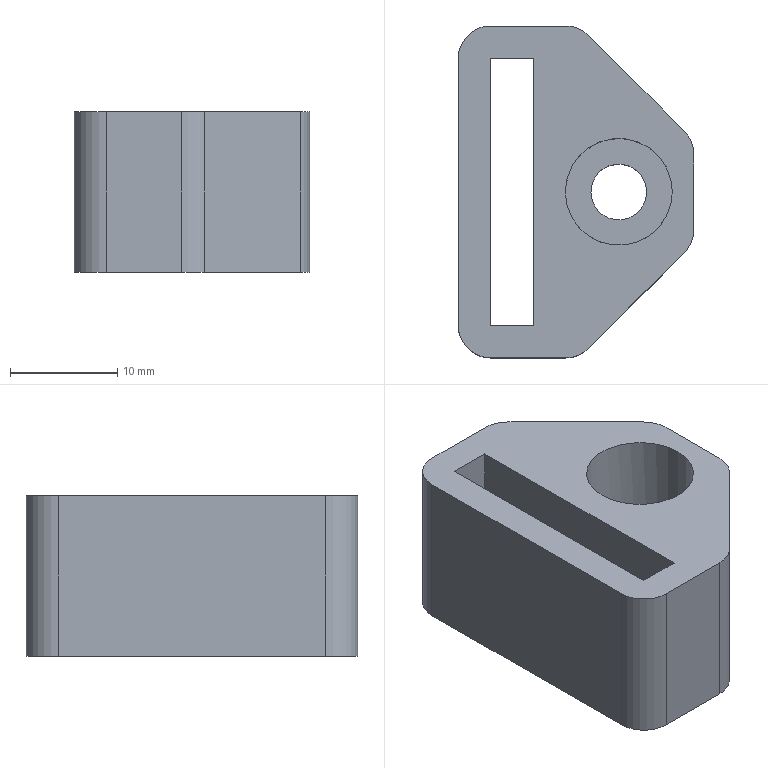Part | NX | features DIE-22 2 | 1 solid | 29 faces | box 22 x 31 x 15 mm | volume 6039 mm3 | plane 17 | cylinder 12 | commonest cylinder face diameters 6 x6 2 x4 5.206 x1 10 x1
STEP:
#1=CARTESIAN_POINT('',(2442.31,-889.273,858.716));
#2=VERTEX_POINT('',#1);
#3=CARTESIAN_POINT('',(2442.31,-864.273,858.716));
#4=VERTEX_POINT('',#3);
#5=CARTESIAN_POINT('',(2442.31,-876.773,858.716));
#6=DIRECTION('',(0.,1.,0.));
#7=VECTOR('',#6,1000.);
#8=LINE('',#5,#7);
#9=EDGE_CURVE('',#2,#4,#8,.T.);
#10=ORIENTED_EDGE('',*,*,#9,.T.);
#11=CARTESIAN_POINT('',(2442.31,-864.273,843.716));
#12=VERTEX_POINT('',#11);
#13=CARTESIAN_POINT('',(2442.31,-864.273,840.716));
#14=DIRECTION('',(0.,0.,1.));
#15=VECTOR('',#14,1000.);
#16=LINE('',#13,#15);
#17=EDGE_CURVE('',#4,#12,#16,.F.);
#18=ORIENTED_EDGE('',*,*,#17,.T.);
#19=CARTESIAN_POINT('',(2442.31,-889.273,843.716));
#20=VERTEX_POINT('',#19);
#21=CARTESIAN_POINT('',(2442.31,-876.773,843.716));
#22=DIRECTION('',(0.,-1.,0.));
#23=VECTOR('',#22,1000.);
#24=LINE('',#21,#23);
#25=EDGE_CURVE('',#12,#20,#24,.T.);
#26=ORIENTED_EDGE('',*,*,#25,.T.);
#27=CARTESIAN_POINT('',(2442.31,-889.273,840.716));
#28=DIRECTION('',(0.,0.,1.));
#29=VECTOR('',#28,1000.);
#30=LINE('',#27,#29);
#31=EDGE_CURVE('',#20,#2,#30,.T.);
#32=ORIENTED_EDGE('',*,*,#31,.T.);
#33=EDGE_LOOP('',(#10,#18,#26,#32));
#34=FACE_BOUND('',#33,.T.);
#35=CARTESIAN_POINT('',(2442.31,-876.773,840.716));
#36=DIRECTION('',(-1.,0.,0.));
#37=DIRECTION('',(0.,0.,1.));
#38=AXIS2_PLACEMENT_3D('',#35,#36,#37);
#39=PLANE('',#38);
#40=ADVANCED_FACE('',(#34),#39,.T.);
#41=CARTESIAN_POINT('',(2445.31,-892.273,843.716));
#42=VERTEX_POINT('',#41);
#43=CARTESIAN_POINT('',(2445.31,-889.273,843.716));
#44=DIRECTION('',(0.,0.,-1.));
#45=DIRECTION('',(-1.,0.,0.));
#46=AXIS2_PLACEMENT_3D('',#43,#44,#45);
#47=CIRCLE('',#46,3.);
#48=EDGE_CURVE('',#42,#20,#47,.T.);
#49=ORIENTED_EDGE('',*,*,#48,.F.);
#50=CARTESIAN_POINT('',(2445.31,-892.273,858.716));
#51=VERTEX_POINT('',#50);
#52=CARTESIAN_POINT('',(2445.31,-892.273,840.716));
#53=DIRECTION('',(0.,0.,1.));
#54=VECTOR('',#53,1000.);
#55=LINE('',#52,#54);
#56=EDGE_CURVE('',#51,#42,#55,.F.);
#57=ORIENTED_EDGE('',*,*,#56,.F.);
#58=CARTESIAN_POINT('',(2445.31,-889.273,858.716));
#59=DIRECTION('',(0.,0.,1.));
#60=DIRECTION('',(1.,0.,0.));
#61=AXIS2_PLACEMENT_3D('',#58,#59,#60);
#62=CIRCLE('',#61,3.);
#63=EDGE_CURVE('',#2,#51,#62,.T.);
#64=ORIENTED_EDGE('',*,*,#63,.F.);
#65=ORIENTED_EDGE('',*,*,#31,.F.);
#66=EDGE_LOOP('',(#49,#57,#64,#65));
#67=FACE_BOUND('',#66,.T.);
#68=CARTESIAN_POINT('',(2445.31,-889.273,840.716));
#69=DIRECTION('',(0.,0.,1.));
#70=DIRECTION('',(1.,0.,0.));
#71=AXIS2_PLACEMENT_3D('',#68,#69,#70);
#72=CYLINDRICAL_SURFACE('',#71,3.);
#73=ADVANCED_FACE('',(#67),#72,.T.);
#74=CARTESIAN_POINT('',(2445.31,-861.273,843.716));
#75=VERTEX_POINT('',#74);
#76=CARTESIAN_POINT('',(2445.31,-864.273,843.716));
#77=DIRECTION('',(0.,0.,-1.));
#78=DIRECTION('',(-1.,0.,0.));
#79=AXIS2_PLACEMENT_3D('',#76,#77,#78);
#80=CIRCLE('',#79,3.);
#81=EDGE_CURVE('',#12,#75,#80,.T.);
#82=ORIENTED_EDGE('',*,*,#81,.F.);
#83=ORIENTED_EDGE('',*,*,#17,.F.);
#84=CARTESIAN_POINT('',(2445.31,-861.273,858.716));
#85=VERTEX_POINT('',#84);
#86=CARTESIAN_POINT('',(2445.31,-864.273,858.716));
#87=DIRECTION('',(0.,0.,1.));
#88=DIRECTION('',(1.,0.,0.));
#89=AXIS2_PLACEMENT_3D('',#86,#87,#88);
#90=CIRCLE('',#89,3.);
#91=EDGE_CURVE('',#85,#4,#90,.T.);
#92=ORIENTED_EDGE('',*,*,#91,.F.);
#93=CARTESIAN_POINT('',(2445.31,-861.273,840.716));
#94=DIRECTION('',(0.,0.,1.));
#95=VECTOR('',#94,1000.);
#96=LINE('',#93,#95);
#97=EDGE_CURVE('',#75,#85,#96,.T.);
#98=ORIENTED_EDGE('',*,*,#97,.F.);
#99=EDGE_LOOP('',(#82,#83,#92,#98));
#100=FACE_BOUND('',#99,.T.);
#101=CARTESIAN_POINT('',(2445.31,-864.273,840.716));
#102=DIRECTION('',(0.,0.,1.));
#103=DIRECTION('',(1.,0.,0.));
#104=AXIS2_PLACEMENT_3D('',#101,#102,#103);
#105=CYLINDRICAL_SURFACE('',#104,3.);
#106=ADVANCED_FACE('',(#100),#105,.T.);
#107=CARTESIAN_POINT('',(2445.31,-864.273,858.716));
#108=VERTEX_POINT('',#107);
#109=CARTESIAN_POINT('',(2445.31,-889.273,858.716));
#110=VERTEX_POINT('',#109);
#111=CARTESIAN_POINT('',(2445.31,-885.523,858.716));
#112=DIRECTION('',(0.,-1.,0.));
#113=VECTOR('',#112,1000.);
#114=LINE('',#111,#113);
#115=EDGE_CURVE('',#108,#110,#114,.T.);
#116=ORIENTED_EDGE('',*,*,#115,.T.);
#117=CARTESIAN_POINT('',(2445.31,-889.273,843.716));
#118=VERTEX_POINT('',#117);
#119=CARTESIAN_POINT('',(2445.31,-889.273,858.516));
#120=DIRECTION('',(0.,0.,-1.));
#121=VECTOR('',#120,1000.);
#122=LINE('',#119,#121);
#123=EDGE_CURVE('',#118,#110,#122,.F.);
#124=ORIENTED_EDGE('',*,*,#123,.F.);
#125=CARTESIAN_POINT('',(2445.31,-864.273,843.716));
#126=VERTEX_POINT('',#125);
#127=CARTESIAN_POINT('',(2445.31,-884.898,843.716));
#128=DIRECTION('',(0.,-1.,0.));
#129=VECTOR('',#128,1000.);
#130=LINE('',#127,#129);
#131=EDGE_CURVE('',#126,#118,#130,.T.);
#132=ORIENTED_EDGE('',*,*,#131,.F.);
#133=CARTESIAN_POINT('',(2445.31,-864.273,858.516));
#134=DIRECTION('',(0.,0.,-1.));
#135=VECTOR('',#134,1000.);
#136=LINE('',#133,#135);
#137=EDGE_CURVE('',#108,#126,#136,.T.);
#138=ORIENTED_EDGE('',*,*,#137,.F.);
#139=EDGE_LOOP('',(#116,#124,#132,#138));
#140=FACE_BOUND('',#139,.T.);
#141=CARTESIAN_POINT('',(2445.31,-884.898,858.516));
#142=DIRECTION('',(1.,0.,0.));
#143=DIRECTION('',(0.,0.,1.));
#144=AXIS2_PLACEMENT_3D('',#141,#142,#143);
#145=PLANE('',#144);
#146=ADVANCED_FACE('',(#140),#145,.T.);
#147=CARTESIAN_POINT('',(2448.31,-889.273,843.716));
#148=VERTEX_POINT('',#147);
#149=CARTESIAN_POINT('',(2448.31,-889.273,846.716));
#150=VERTEX_POINT('',#149);
#151=CARTESIAN_POINT('',(2448.31,-889.273,858.516));
#152=DIRECTION('',(0.,0.,1.));
#153=VECTOR('',#152,1000.);
#154=LINE('',#151,#153);
#155=EDGE_CURVE('',#148,#150,#154,.T.);
#156=ORIENTED_EDGE('',*,*,#155,.F.);
#157=CARTESIAN_POINT('',(2448.697,-889.273,843.716));
#158=DIRECTION('',(1.,0.,0.));
#159=VECTOR('',#158,1000.);
#160=LINE('',#157,#159);
#161=EDGE_CURVE('',#118,#148,#160,.T.);
#162=ORIENTED_EDGE('',*,*,#161,.F.);
#163=ORIENTED_EDGE('',*,*,#123,.T.);
#164=CARTESIAN_POINT('',(2449.31,-889.273,858.716));
#165=VERTEX_POINT('',#164);
#166=CARTESIAN_POINT('',(2447.31,-889.273,858.716));
#167=DIRECTION('',(1.,0.,0.));
#168=VECTOR('',#167,1000.);
#169=LINE('',#166,#168);
#170=EDGE_CURVE('',#165,#110,#169,.F.);
#171=ORIENTED_EDGE('',*,*,#170,.F.);
#172=CARTESIAN_POINT('',(2449.31,-889.273,846.716));
#173=VERTEX_POINT('',#172);
#174=CARTESIAN_POINT('',(2449.31,-889.273,858.516));
#175=DIRECTION('',(0.,0.,1.));
#176=VECTOR('',#175,1000.);
#177=LINE('',#174,#176);
#178=EDGE_CURVE('',#173,#165,#177,.T.);
#179=ORIENTED_EDGE('',*,*,#178,.F.);
#180=CARTESIAN_POINT('',(2449.81,-889.273,846.716));
#181=DIRECTION('',(-1.,0.,0.));
#182=VECTOR('',#181,1000.);
#183=LINE('',#180,#182);
#184=EDGE_CURVE('',#173,#150,#183,.T.);
#185=ORIENTED_EDGE('',*,*,#184,.T.);
#186=EDGE_LOOP('',(#156,#162,#163,#171,#179,#185));
#187=FACE_BOUND('',#186,.T.);
#188=CARTESIAN_POINT('',(2448.697,-889.273,858.516));
#189=DIRECTION('',(0.,1.,0.));
#190=DIRECTION('',(0.,0.,-1.));
#191=AXIS2_PLACEMENT_3D('',#188,#189,#190);
#192=PLANE('',#191);
#193=ADVANCED_FACE('',(#187),#192,.T.);
#194=CARTESIAN_POINT('',(2448.31,-864.273,843.716));
#195=VERTEX_POINT('',#194);
#196=CARTESIAN_POINT('',(2448.697,-864.273,843.716));
#197=DIRECTION('',(-1.,0.,0.));
#198=VECTOR('',#197,1000.);
#199=LINE('',#196,#198);
#200=EDGE_CURVE('',#195,#126,#199,.T.);
#201=ORIENTED_EDGE('',*,*,#200,.F.);
#202=CARTESIAN_POINT('',(2448.31,-864.273,846.716));
#203=VERTEX_POINT('',#202);
#204=CARTESIAN_POINT('',(2448.31,-864.273,858.516));
#205=DIRECTION('',(0.,0.,-1.));
#206=VECTOR('',#205,1000.);
#207=LINE('',#204,#206);
#208=EDGE_CURVE('',#203,#195,#207,.T.);
#209=ORIENTED_EDGE('',*,*,#208,.F.);
#210=CARTESIAN_POINT('',(2449.31,-864.273,846.716));
#211=VERTEX_POINT('',#210);
#212=CARTESIAN_POINT('',(2448.697,-864.273,846.716));
#213=DIRECTION('',(-1.,0.,0.));
#214=VECTOR('',#213,1000.);
#215=LINE('',#212,#214);
#216=EDGE_CURVE('',#211,#203,#215,.T.);
#217=ORIENTED_EDGE('',*,*,#216,.F.);
#218=CARTESIAN_POINT('',(2449.31,-864.273,858.716));
#219=VERTEX_POINT('',#218);
#220=CARTESIAN_POINT('',(2449.31,-864.273,858.516));
#221=DIRECTION('',(0.,0.,-1.));
#222=VECTOR('',#221,1000.);
#223=LINE('',#220,#222);
#224=EDGE_CURVE('',#219,#211,#223,.T.);
#225=ORIENTED_EDGE('',*,*,#224,.F.);
#226=CARTESIAN_POINT('',(2447.31,-864.273,858.716));
#227=DIRECTION('',(1.,0.,0.));
#228=VECTOR('',#227,1000.);
#229=LINE('',#226,#228);
#230=EDGE_CURVE('',#219,#108,#229,.F.);
#231=ORIENTED_EDGE('',*,*,#230,.T.);
#232=ORIENTED_EDGE('',*,*,#137,.T.);
#233=EDGE_LOOP('',(#201,#209,#217,#225,#231,#232));
#234=FACE_BOUND('',#233,.T.);
#235=CARTESIAN_POINT('',(2448.697,-864.273,858.516));
#236=DIRECTION('',(0.,-1.,0.));
#237=DIRECTION('',(0.,0.,-1.));
#238=AXIS2_PLACEMENT_3D('',#235,#236,#237);
#239=PLANE('',#238);
#240=ADVANCED_FACE('',(#234),#239,.T.);
#241=CARTESIAN_POINT('',(2452.36,-861.273,858.716));
#242=VERTEX_POINT('',#241);
#243=CARTESIAN_POINT('',(2447.81,-861.273,858.716));
#244=DIRECTION('',(1.,0.,0.));
#245=VECTOR('',#244,1000.);
#246=LINE('',#243,#245);
#247=EDGE_CURVE('',#85,#242,#246,.T.);
#248=ORIENTED_EDGE('',*,*,#247,.T.);
#249=CARTESIAN_POINT('',(2452.36,-861.273,843.716));
#250=VERTEX_POINT('',#249);
#251=CARTESIAN_POINT('',(2452.36,-861.273,840.716));
#252=DIRECTION('',(0.,0.,1.));
#253=VECTOR('',#252,1000.);
#254=LINE('',#251,#253);
#255=EDGE_CURVE('',#242,#250,#254,.F.);
#256=ORIENTED_EDGE('',*,*,#255,.T.);
#257=CARTESIAN_POINT('',(2447.81,-861.273,843.716));
#258=DIRECTION('',(-1.,0.,0.));
#259=VECTOR('',#258,1000.);
#260=LINE('',#257,#259);
#261=EDGE_CURVE('',#250,#75,#260,.T.);
#262=ORIENTED_EDGE('',*,*,#261,.T.);
#263=ORIENTED_EDGE('',*,*,#97,.T.);
#264=EDGE_LOOP('',(#248,#256,#262,#263));
#265=FACE_BOUND('',#264,.T.);
#266=CARTESIAN_POINT('',(2447.81,-861.273,840.716));
#267=DIRECTION('',(0.,1.,0.));
#268=DIRECTION('',(0.,0.,1.));
#269=AXIS2_PLACEMENT_3D('',#266,#267,#268);
#270=PLANE('',#269);
#271=ADVANCED_FACE('',(#265),#270,.T.);
#272=CARTESIAN_POINT('',(2452.36,-892.273,843.716));
#273=VERTEX_POINT('',#272);
#274=CARTESIAN_POINT('',(2447.81,-892.273,843.716));
#275=DIRECTION('',(1.,0.,0.));
#276=VECTOR('',#275,1000.);
#277=LINE('',#274,#276);
#278=EDGE_CURVE('',#42,#273,#277,.T.);
#279=ORIENTED_EDGE('',*,*,#278,.T.);
#280=CARTESIAN_POINT('',(2452.36,-892.273,858.716));
#281=VERTEX_POINT('',#280);
#282=CARTESIAN_POINT('',(2452.36,-892.273,840.716));
#283=DIRECTION('',(0.,0.,-1.));
#284=VECTOR('',#283,1000.);
#285=LINE('',#282,#284);
#286=EDGE_CURVE('',#273,#281,#285,.F.);
#287=ORIENTED_EDGE('',*,*,#286,.T.);
#288=CARTESIAN_POINT('',(2447.81,-892.273,858.716));
#289=DIRECTION('',(-1.,0.,0.));
#290=VECTOR('',#289,1000.);
#291=LINE('',#288,#290);
#292=EDGE_CURVE('',#281,#51,#291,.T.);
#293=ORIENTED_EDGE('',*,*,#292,.T.);
#294=ORIENTED_EDGE('',*,*,#56,.T.);
#295=EDGE_LOOP('',(#279,#287,#293,#294));
#296=FACE_BOUND('',#295,.T.);
#297=CARTESIAN_POINT('',(2447.81,-892.273,840.716));
#298=DIRECTION('',(0.,-1.,0.));
#299=DIRECTION('',(0.,0.,-1.));
#300=AXIS2_PLACEMENT_3D('',#297,#298,#299);
#301=PLANE('',#300);
#302=ADVANCED_FACE('',(#296),#301,.T.);
#303=ORIENTED_EDGE('',*,*,#161,.T.);
#304=CARTESIAN_POINT('',(2449.31,-890.273,843.716));
#305=VERTEX_POINT('',#304);
#306=CARTESIAN_POINT('',(2449.31,-889.273,843.716));
#307=DIRECTION('',(0.,0.,-1.));
#308=DIRECTION('',(-1.,0.,0.));
#309=AXIS2_PLACEMENT_3D('',#306,#307,#308);
#310=CIRCLE('',#309,1.);
#311=EDGE_CURVE('',#148,#305,#310,.F.);
#312=ORIENTED_EDGE('',*,*,#311,.T.);
#313=CARTESIAN_POINT('',(2449.81,-890.273,843.716));
#314=VERTEX_POINT('',#313);
#315=CARTESIAN_POINT('',(2447.81,-890.273,843.716));
#316=DIRECTION('',(1.,0.,0.));
#317=VECTOR('',#316,1000.);
#318=LINE('',#315,#317);
#319=EDGE_CURVE('',#305,#314,#318,.T.);
#320=ORIENTED_EDGE('',*,*,#319,.T.);
#321=CARTESIAN_POINT('',(2450.81,-889.273,843.716));
#322=VERTEX_POINT('',#321);
#323=CARTESIAN_POINT('',(2449.81,-889.273,843.716));
#324=DIRECTION('',(0.,0.,-1.));
#325=DIRECTION('',(-1.,0.,0.));
#326=AXIS2_PLACEMENT_3D('',#323,#324,#325);
#327=CIRCLE('',#326,1.);
#328=EDGE_CURVE('',#314,#322,#327,.F.);
#329=ORIENTED_EDGE('',*,*,#328,.T.);
#330=CARTESIAN_POINT('',(2450.81,-864.273,843.716));
#331=VERTEX_POINT('',#330);
#332=CARTESIAN_POINT('',(2450.81,-884.898,843.716));
#333=DIRECTION('',(0.,-1.,0.));
#334=VECTOR('',#333,1000.);
#335=LINE('',#332,#334);
#336=EDGE_CURVE('',#331,#322,#335,.T.);
#337=ORIENTED_EDGE('',*,*,#336,.F.);
#338=CARTESIAN_POINT('',(2449.81,-863.273,843.716));
#339=VERTEX_POINT('',#338);
#340=CARTESIAN_POINT('',(2449.81,-864.273,843.716));
#341=DIRECTION('',(0.,0.,-1.));
#342=DIRECTION('',(-1.,0.,0.));
#343=AXIS2_PLACEMENT_3D('',#340,#341,#342);
#344=CIRCLE('',#343,1.);
#345=EDGE_CURVE('',#331,#339,#344,.F.);
#346=ORIENTED_EDGE('',*,*,#345,.T.);
#347=CARTESIAN_POINT('',(2449.31,-863.273,843.716));
#348=VERTEX_POINT('',#347);
#349=CARTESIAN_POINT('',(2447.81,-863.273,843.716));
#350=DIRECTION('',(-1.,0.,0.));
#351=VECTOR('',#350,1000.);
#352=LINE('',#349,#351);
#353=EDGE_CURVE('',#339,#348,#352,.T.);
#354=ORIENTED_EDGE('',*,*,#353,.T.);
#355=CARTESIAN_POINT('',(2449.31,-864.273,843.716));
#356=DIRECTION('',(0.,0.,-1.));
#357=DIRECTION('',(-1.,0.,0.));
#358=AXIS2_PLACEMENT_3D('',#355,#356,#357);
#359=CIRCLE('',#358,1.);
#360=EDGE_CURVE('',#348,#195,#359,.F.);
#361=ORIENTED_EDGE('',*,*,#360,.T.);
#362=ORIENTED_EDGE('',*,*,#200,.T.);
#363=ORIENTED_EDGE('',*,*,#131,.T.);
#364=EDGE_LOOP('',(#303,#312,#320,#329,#337,#346,#354,#361,#362,#363));
#365=FACE_BOUND('',#364,.T.);
#366=CARTESIAN_POINT('',(2454.481,-891.395,843.716));
#367=VERTEX_POINT('',#366);
#368=CARTESIAN_POINT('',(2452.36,-889.273,843.716));
#369=DIRECTION('',(0.,0.,-1.));
#370=DIRECTION('',(-1.,0.,0.));
#371=AXIS2_PLACEMENT_3D('',#368,#369,#370);
#372=CIRCLE('',#371,3.);
#373=EDGE_CURVE('',#367,#273,#372,.T.);
#374=ORIENTED_EDGE('',*,*,#373,.T.);
#375=ORIENTED_EDGE('',*,*,#278,.F.);
#376=ORIENTED_EDGE('',*,*,#48,.T.);
#377=ORIENTED_EDGE('',*,*,#25,.F.);
#378=ORIENTED_EDGE('',*,*,#81,.T.);
#379=ORIENTED_EDGE('',*,*,#261,.F.);
#380=CARTESIAN_POINT('',(2454.481,-862.152,843.716));
#381=VERTEX_POINT('',#380);
#382=CARTESIAN_POINT('',(2452.36,-864.273,843.716));
#383=DIRECTION('',(0.,0.,-1.));
#384=DIRECTION('',(-1.,0.,0.));
#385=AXIS2_PLACEMENT_3D('',#382,#383,#384);
#386=CIRCLE('',#385,3.);
#387=EDGE_CURVE('',#250,#381,#386,.T.);
#388=ORIENTED_EDGE('',*,*,#387,.T.);
#389=CARTESIAN_POINT('',(2463.431,-871.102,843.716));
#390=VERTEX_POINT('',#389);
#391=CARTESIAN_POINT('',(2458.456,-866.127,843.716));
#392=DIRECTION('',(-0.7071,0.7071,0.));
#393=VECTOR('',#392,1000.);
#394=LINE('',#391,#393);
#395=EDGE_CURVE('',#381,#390,#394,.F.);
#396=ORIENTED_EDGE('',*,*,#395,.T.);
#397=CARTESIAN_POINT('',(2464.31,-873.223,843.716));
#398=VERTEX_POINT('',#397);
#399=CARTESIAN_POINT('',(2461.31,-873.223,843.716));
#400=DIRECTION('',(0.,0.,-1.));
#401=DIRECTION('',(-1.,0.,0.));
#402=AXIS2_PLACEMENT_3D('',#399,#400,#401);
#403=CIRCLE('',#402,3.);
#404=EDGE_CURVE('',#390,#398,#403,.T.);
#405=ORIENTED_EDGE('',*,*,#404,.T.);
#406=CARTESIAN_POINT('',(2464.31,-880.324,843.716));
#407=VERTEX_POINT('',#406);
#408=CARTESIAN_POINT('',(2464.31,-876.773,843.716));
#409=DIRECTION('',(0.,1.,0.));
#410=VECTOR('',#409,1000.);
#411=LINE('',#408,#410);
#412=EDGE_CURVE('',#407,#398,#411,.T.);
#413=ORIENTED_EDGE('',*,*,#412,.F.);
#414=CARTESIAN_POINT('',(2463.431,-882.445,843.716));
#415=VERTEX_POINT('',#414);
#416=CARTESIAN_POINT('',(2461.31,-880.324,843.716));
#417=DIRECTION('',(0.,0.,-1.));
#418=DIRECTION('',(-1.,0.,0.));
#419=AXIS2_PLACEMENT_3D('',#416,#417,#418);
#420=CIRCLE('',#419,3.);
#421=EDGE_CURVE('',#407,#415,#420,.T.);
#422=ORIENTED_EDGE('',*,*,#421,.T.);
#423=CARTESIAN_POINT('',(2458.456,-887.42,843.716));
#424=DIRECTION('',(0.7071,0.7071,0.));
#425=VECTOR('',#424,1000.);
#426=LINE('',#423,#425);
#427=EDGE_CURVE('',#415,#367,#426,.F.);
#428=ORIENTED_EDGE('',*,*,#427,.T.);
#429=EDGE_LOOP('',(#374,#375,#376,#377,#378,#379,#388,#396,#405,#413,#422,#428));
#430=FACE_BOUND('',#429,.T.);
#431=CARTESIAN_POINT('',(2454.707,-876.773,843.716));
#432=VERTEX_POINT('',#431);
#433=CARTESIAN_POINT('',(2457.31,-876.773,843.716));
#434=DIRECTION('',(0.,0.,-1.));
#435=DIRECTION('',(-1.,0.,0.));
#436=AXIS2_PLACEMENT_3D('',#433,#434,#435);
#437=CIRCLE('',#436,2.603);
#438=EDGE_CURVE('',#432,#432,#437,.T.);
#439=ORIENTED_EDGE('',*,*,#438,.F.);
#440=EDGE_LOOP('',(#439));
#441=FACE_BOUND('',#440,.T.);
#442=CARTESIAN_POINT('',(2447.81,-876.773,843.716));
#443=DIRECTION('',(0.,0.,-1.));
#444=DIRECTION('',(-1.,0.,0.));
#445=AXIS2_PLACEMENT_3D('',#442,#443,#444);
#446=PLANE('',#445);
#447=ADVANCED_FACE('',(#365,#430,#441),#446,.T.);
#448=ORIENTED_EDGE('',*,*,#230,.F.);
#449=CARTESIAN_POINT('',(2449.31,-876.773,858.716));
#450=DIRECTION('',(0.,-1.,0.));
#451=VECTOR('',#450,1000.);
#452=LINE('',#449,#451);
#453=EDGE_CURVE('',#165,#219,#452,.F.);
#454=ORIENTED_EDGE('',*,*,#453,.F.);
#455=ORIENTED_EDGE('',*,*,#170,.T.);
#456=ORIENTED_EDGE('',*,*,#115,.F.);
#457=EDGE_LOOP('',(#448,#454,#455,#456));
#458=FACE_BOUND('',#457,.T.);
#459=CARTESIAN_POINT('',(2454.481,-862.152,858.716));
#460=VERTEX_POINT('',#459);
#461=CARTESIAN_POINT('',(2452.36,-864.273,858.716));
#462=DIRECTION('',(0.,0.,1.));
#463=DIRECTION('',(1.,0.,0.));
#464=AXIS2_PLACEMENT_3D('',#461,#462,#463);
#465=CIRCLE('',#464,3.);
#466=EDGE_CURVE('',#460,#242,#465,.T.);
#467=ORIENTED_EDGE('',*,*,#466,.T.);
#468=ORIENTED_EDGE('',*,*,#247,.F.);
#469=ORIENTED_EDGE('',*,*,#91,.T.);
#470=ORIENTED_EDGE('',*,*,#9,.F.);
#471=ORIENTED_EDGE('',*,*,#63,.T.);
#472=ORIENTED_EDGE('',*,*,#292,.F.);
#473=CARTESIAN_POINT('',(2454.481,-891.395,858.716));
#474=VERTEX_POINT('',#473);
#475=CARTESIAN_POINT('',(2452.36,-889.273,858.716));
#476=DIRECTION('',(0.,0.,1.));
#477=DIRECTION('',(1.,0.,0.));
#478=AXIS2_PLACEMENT_3D('',#475,#476,#477);
#479=CIRCLE('',#478,3.);
#480=EDGE_CURVE('',#281,#474,#479,.T.);
#481=ORIENTED_EDGE('',*,*,#480,.T.);
#482=CARTESIAN_POINT('',(2463.431,-882.445,858.716));
#483=VERTEX_POINT('',#482);
#484=CARTESIAN_POINT('',(2458.456,-887.42,858.716));
#485=DIRECTION('',(-0.7071,-0.7071,0.));
#486=VECTOR('',#485,1000.);
#487=LINE('',#484,#486);
#488=EDGE_CURVE('',#474,#483,#487,.F.);
#489=ORIENTED_EDGE('',*,*,#488,.T.);
#490=CARTESIAN_POINT('',(2464.31,-880.324,858.716));
#491=VERTEX_POINT('',#490);
#492=CARTESIAN_POINT('',(2461.31,-880.324,858.716));
#493=DIRECTION('',(0.,0.,1.));
#494=DIRECTION('',(1.,0.,0.));
#495=AXIS2_PLACEMENT_3D('',#492,#493,#494);
#496=CIRCLE('',#495,3.);
#497=EDGE_CURVE('',#483,#491,#496,.T.);
#498=ORIENTED_EDGE('',*,*,#497,.T.);
#499=CARTESIAN_POINT('',(2464.31,-873.223,858.716));
#500=VERTEX_POINT('',#499);
#501=CARTESIAN_POINT('',(2464.31,-876.773,858.716));
#502=DIRECTION('',(0.,-1.,0.));
#503=VECTOR('',#502,1000.);
#504=LINE('',#501,#503);
#505=EDGE_CURVE('',#500,#491,#504,.T.);
#506=ORIENTED_EDGE('',*,*,#505,.F.);
#507=CARTESIAN_POINT('',(2463.431,-871.102,858.716));
#508=VERTEX_POINT('',#507);
#509=CARTESIAN_POINT('',(2461.31,-873.223,858.716));
#510=DIRECTION('',(0.,0.,1.));
#511=DIRECTION('',(1.,0.,0.));
#512=AXIS2_PLACEMENT_3D('',#509,#510,#511);
#513=CIRCLE('',#512,3.);
#514=EDGE_CURVE('',#500,#508,#513,.T.);
#515=ORIENTED_EDGE('',*,*,#514,.T.);
#516=CARTESIAN_POINT('',(2458.456,-866.127,858.716));
#517=DIRECTION('',(0.7071,-0.7071,0.));
#518=VECTOR('',#517,1000.);
#519=LINE('',#516,#518);
#520=EDGE_CURVE('',#508,#460,#519,.F.);
#521=ORIENTED_EDGE('',*,*,#520,.T.);
#522=EDGE_LOOP('',(#467,#468,#469,#470,#471,#472,#481,#489,#498,#506,#515,#521));
#523=FACE_BOUND('',#522,.T.);
#524=CARTESIAN_POINT('',(2462.31,-876.773,858.716));
#525=VERTEX_POINT('',#524);
#526=CARTESIAN_POINT('',(2457.31,-876.773,858.716));
#527=DIRECTION('',(0.,0.,1.));
#528=DIRECTION('',(1.,0.,0.));
#529=AXIS2_PLACEMENT_3D('',#526,#527,#528);
#530=CIRCLE('',#529,5.);
#531=EDGE_CURVE('',#525,#525,#530,.T.);
#532=ORIENTED_EDGE('',*,*,#531,.F.);
#533=EDGE_LOOP('',(#532));
#534=FACE_BOUND('',#533,.T.);
#535=CARTESIAN_POINT('',(2447.81,-876.773,858.716));
#536=DIRECTION('',(0.,0.,1.));
#537=DIRECTION('',(1.,0.,0.));
#538=AXIS2_PLACEMENT_3D('',#535,#536,#537);
#539=PLANE('',#538);
#540=ADVANCED_FACE('',(#458,#523,#534),#539,.T.);
#541=ORIENTED_EDGE('',*,*,#319,.F.);
#542=CARTESIAN_POINT('',(2449.31,-890.273,846.716));
#543=VERTEX_POINT('',#542);
#544=CARTESIAN_POINT('',(2449.31,-890.273,858.516));
#545=DIRECTION('',(0.,0.,-1.));
#546=VECTOR('',#545,1000.);
#547=LINE('',#544,#546);
#548=EDGE_CURVE('',#305,#543,#547,.F.);
#549=ORIENTED_EDGE('',*,*,#548,.T.);
#550=CARTESIAN_POINT('',(2449.81,-890.273,846.716));
#551=VERTEX_POINT('',#550);
#552=CARTESIAN_POINT('',(2449.81,-890.273,846.716));
#553=DIRECTION('',(-1.,0.,0.));
#554=VECTOR('',#553,1000.);
#555=LINE('',#552,#554);
#556=EDGE_CURVE('',#551,#543,#555,.T.);
#557=ORIENTED_EDGE('',*,*,#556,.F.);
#558=CARTESIAN_POINT('',(2449.81,-890.273,843.716));
#559=DIRECTION('',(0.,0.,1.));
#560=VECTOR('',#559,1000.);
#561=LINE('',#558,#560);
#562=EDGE_CURVE('',#551,#314,#561,.F.);
#563=ORIENTED_EDGE('',*,*,#562,.T.);
#564=EDGE_LOOP('',(#541,#549,#557,#563));
#565=FACE_BOUND('',#564,.T.);
#566=CARTESIAN_POINT('',(2448.697,-890.273,858.516));
#567=DIRECTION('',(0.,1.,0.));
#568=DIRECTION('',(0.,0.,-1.));
#569=AXIS2_PLACEMENT_3D('',#566,#567,#568);
#570=PLANE('',#569);
#571=ADVANCED_FACE('',(#565),#570,.T.);
#572=CARTESIAN_POINT('',(2449.31,-863.273,846.716));
#573=VERTEX_POINT('',#572);
#574=CARTESIAN_POINT('',(2449.81,-863.273,846.716));
#575=VERTEX_POINT('',#574);
#576=CARTESIAN_POINT('',(2449.81,-863.273,846.716));
#577=DIRECTION('',(1.,0.,0.));
#578=VECTOR('',#577,1000.);
#579=LINE('',#576,#578);
#580=EDGE_CURVE('',#573,#575,#579,.T.);
#581=ORIENTED_EDGE('',*,*,#580,.F.);
#582=CARTESIAN_POINT('',(2449.31,-863.273,858.516));
#583=DIRECTION('',(0.,0.,1.));
#584=VECTOR('',#583,1000.);
#585=LINE('',#582,#584);
#586=EDGE_CURVE('',#573,#348,#585,.F.);
#587=ORIENTED_EDGE('',*,*,#586,.T.);
#588=ORIENTED_EDGE('',*,*,#353,.F.);
#589=CARTESIAN_POINT('',(2449.81,-863.273,846.716));
#590=DIRECTION('',(0.,0.,-1.));
#591=VECTOR('',#590,1000.);
#592=LINE('',#589,#591);
#593=EDGE_CURVE('',#339,#575,#592,.F.);
#594=ORIENTED_EDGE('',*,*,#593,.T.);
#595=EDGE_LOOP('',(#581,#587,#588,#594));
#596=FACE_BOUND('',#595,.T.);
#597=CARTESIAN_POINT('',(2448.697,-863.273,858.516));
#598=DIRECTION('',(0.,-1.,0.));
#599=DIRECTION('',(0.,0.,-1.));
#600=AXIS2_PLACEMENT_3D('',#597,#598,#599);
#601=PLANE('',#600);
#602=ADVANCED_FACE('',(#596),#601,.T.);
#603=ORIENTED_EDGE('',*,*,#412,.T.);
#604=CARTESIAN_POINT('',(2464.31,-873.223,840.716));
#605=DIRECTION('',(0.,0.,-1.));
#606=VECTOR('',#605,1000.);
#607=LINE('',#604,#606);
#608=EDGE_CURVE('',#398,#500,#607,.F.);
#609=ORIENTED_EDGE('',*,*,#608,.T.);
#610=ORIENTED_EDGE('',*,*,#505,.T.);
#611=CARTESIAN_POINT('',(2464.31,-880.324,840.716));
#612=DIRECTION('',(0.,0.,1.));
#613=VECTOR('',#612,1000.);
#614=LINE('',#611,#613);
#615=EDGE_CURVE('',#491,#407,#614,.F.);
#616=ORIENTED_EDGE('',*,*,#615,.T.);
#617=EDGE_LOOP('',(#603,#609,#610,#616));
#618=FACE_BOUND('',#617,.T.);
#619=CARTESIAN_POINT('',(2464.31,-876.773,840.716));
#620=DIRECTION('',(1.,0.,0.));
#621=DIRECTION('',(0.,0.,-1.));
#622=AXIS2_PLACEMENT_3D('',#619,#620,#621);
#623=PLANE('',#622);
#624=ADVANCED_FACE('',(#618),#623,.T.);
#625=ORIENTED_EDGE('',*,*,#438,.T.);
#626=EDGE_LOOP('',(#625));
#627=FACE_BOUND('',#626,.T.);
#628=CARTESIAN_POINT('',(2459.913,-876.773,850.716));
#629=VERTEX_POINT('',#628);
#630=CARTESIAN_POINT('',(2457.31,-876.773,850.716));
#631=DIRECTION('',(0.,0.,1.));
#632=DIRECTION('',(1.,0.,0.));
#633=AXIS2_PLACEMENT_3D('',#630,#631,#632);
#634=CIRCLE('',#633,2.603);
#635=EDGE_CURVE('',#629,#629,#634,.T.);
#636=ORIENTED_EDGE('',*,*,#635,.T.);
#637=EDGE_LOOP('',(#636));
#638=FACE_BOUND('',#637,.T.);
#639=CARTESIAN_POINT('',(2457.31,-876.773,842.716));
#640=DIRECTION('',(0.,0.,1.));
#641=DIRECTION('',(1.,0.,0.));
#642=AXIS2_PLACEMENT_3D('',#639,#640,#641);
#643=CYLINDRICAL_SURFACE('',#642,2.603);
#644=ADVANCED_FACE('',(#627,#638),#643,.F.);
#645=ORIENTED_EDGE('',*,*,#531,.T.);
#646=EDGE_LOOP('',(#645));
#647=FACE_BOUND('',#646,.T.);
#648=CARTESIAN_POINT('',(2457.31,-871.773,850.716));
#649=VERTEX_POINT('',#648);
#650=CARTESIAN_POINT('',(2457.31,-876.773,850.716));
#651=DIRECTION('',(0.,0.,1.));
#652=DIRECTION('',(0.,1.,0.));
#653=AXIS2_PLACEMENT_3D('',#650,#651,#652);
#654=CIRCLE('',#653,5.);
#655=EDGE_CURVE('',#649,#649,#654,.F.);
#656=ORIENTED_EDGE('',*,*,#655,.T.);
#657=EDGE_LOOP('',(#656));
#658=FACE_BOUND('',#657,.T.);
#659=CARTESIAN_POINT('',(2457.31,-876.773,850.716));
#660=DIRECTION('',(0.,0.,1.));
#661=DIRECTION('',(1.,0.,0.));
#662=AXIS2_PLACEMENT_3D('',#659,#660,#661);
#663=CYLINDRICAL_SURFACE('',#662,5.);
#664=ADVANCED_FACE('',(#647,#658),#663,.F.);
#665=ORIENTED_EDGE('',*,*,#635,.F.);
#666=EDGE_LOOP('',(#665));
#667=FACE_BOUND('',#666,.T.);
#668=ORIENTED_EDGE('',*,*,#655,.F.);
#669=EDGE_LOOP('',(#668));
#670=FACE_BOUND('',#669,.T.);
#671=CARTESIAN_POINT('',(2457.31,-876.773,850.716));
#672=DIRECTION('',(0.,0.,1.));
#673=DIRECTION('',(1.,0.,0.));
#674=AXIS2_PLACEMENT_3D('',#671,#672,#673);
#675=PLANE('',#674);
#676=ADVANCED_FACE('',(#667,#670),#675,.T.);
#677=ORIENTED_EDGE('',*,*,#395,.F.);
#678=CARTESIAN_POINT('',(2454.481,-862.152,840.716));
#679=DIRECTION('',(0.,0.,-1.));
#680=VECTOR('',#679,1000.);
#681=LINE('',#678,#680);
#682=EDGE_CURVE('',#381,#460,#681,.F.);
#683=ORIENTED_EDGE('',*,*,#682,.T.);
#684=ORIENTED_EDGE('',*,*,#520,.F.);
#685=CARTESIAN_POINT('',(2463.431,-871.102,840.716));
#686=DIRECTION('',(0.,0.,1.));
#687=VECTOR('',#686,1000.);
#688=LINE('',#685,#687);
#689=EDGE_CURVE('',#508,#390,#688,.F.);
#690=ORIENTED_EDGE('',*,*,#689,.T.);
#691=EDGE_LOOP('',(#677,#683,#684,#690));
#692=FACE_BOUND('',#691,.T.);
#693=CARTESIAN_POINT('',(2463.956,-871.627,840.716));
#694=DIRECTION('',(-0.7071,-0.7071,0.));
#695=DIRECTION('',(0.,0.,1.));
#696=AXIS2_PLACEMENT_3D('',#693,#694,#695);
#697=PLANE('',#696);
#698=ADVANCED_FACE('',(#692),#697,.F.);
#699=ORIENTED_EDGE('',*,*,#427,.F.);
#700=CARTESIAN_POINT('',(2463.431,-882.445,840.716));
#701=DIRECTION('',(0.,0.,-1.));
#702=VECTOR('',#701,1000.);
#703=LINE('',#700,#702);
#704=EDGE_CURVE('',#415,#483,#703,.F.);
#705=ORIENTED_EDGE('',*,*,#704,.T.);
#706=ORIENTED_EDGE('',*,*,#488,.F.);
#707=CARTESIAN_POINT('',(2454.481,-891.395,840.716));
#708=DIRECTION('',(0.,0.,1.));
#709=VECTOR('',#708,1000.);
#710=LINE('',#707,#709);
#711=EDGE_CURVE('',#474,#367,#710,.F.);
#712=ORIENTED_EDGE('',*,*,#711,.T.);
#713=EDGE_LOOP('',(#699,#705,#706,#712));
#714=FACE_BOUND('',#713,.T.);
#715=CARTESIAN_POINT('',(2453.956,-891.92,840.716));
#716=DIRECTION('',(-0.7071,0.7071,0.));
#717=DIRECTION('',(0.,0.,1.));
#718=AXIS2_PLACEMENT_3D('',#715,#716,#717);
#719=PLANE('',#718);
#720=ADVANCED_FACE('',(#714),#719,.F.);
#721=ORIENTED_EDGE('',*,*,#466,.F.);
#722=ORIENTED_EDGE('',*,*,#682,.F.);
#723=ORIENTED_EDGE('',*,*,#387,.F.);
#724=ORIENTED_EDGE('',*,*,#255,.F.);
#725=EDGE_LOOP('',(#721,#722,#723,#724));
#726=FACE_BOUND('',#725,.T.);
#727=CARTESIAN_POINT('',(2452.36,-864.273,840.716));
#728=DIRECTION('',(0.,0.,1.));
#729=DIRECTION('',(1.,0.,0.));
#730=AXIS2_PLACEMENT_3D('',#727,#728,#729);
#731=CYLINDRICAL_SURFACE('',#730,3.);
#732=ADVANCED_FACE('',(#726),#731,.T.);
#733=ORIENTED_EDGE('',*,*,#404,.F.);
#734=ORIENTED_EDGE('',*,*,#689,.F.);
#735=ORIENTED_EDGE('',*,*,#514,.F.);
#736=ORIENTED_EDGE('',*,*,#608,.F.);
#737=EDGE_LOOP('',(#733,#734,#735,#736));
#738=FACE_BOUND('',#737,.T.);
#739=CARTESIAN_POINT('',(2461.31,-873.223,840.716));
#740=DIRECTION('',(0.,0.,-1.));
#741=DIRECTION('',(-1.,0.,0.));
#742=AXIS2_PLACEMENT_3D('',#739,#740,#741);
#743=CYLINDRICAL_SURFACE('',#742,3.);
#744=ADVANCED_FACE('',(#738),#743,.T.);
#745=ORIENTED_EDGE('',*,*,#497,.F.);
#746=ORIENTED_EDGE('',*,*,#704,.F.);
#747=ORIENTED_EDGE('',*,*,#421,.F.);
#748=ORIENTED_EDGE('',*,*,#615,.F.);
#749=EDGE_LOOP('',(#745,#746,#747,#748));
#750=FACE_BOUND('',#749,.T.);
#751=CARTESIAN_POINT('',(2461.31,-880.324,840.716));
#752=DIRECTION('',(0.,0.,1.));
#753=DIRECTION('',(1.,0.,0.));
#754=AXIS2_PLACEMENT_3D('',#751,#752,#753);
#755=CYLINDRICAL_SURFACE('',#754,3.);
#756=ADVANCED_FACE('',(#750),#755,.T.);
#757=ORIENTED_EDGE('',*,*,#373,.F.);
#758=ORIENTED_EDGE('',*,*,#711,.F.);
#759=ORIENTED_EDGE('',*,*,#480,.F.);
#760=ORIENTED_EDGE('',*,*,#286,.F.);
#761=EDGE_LOOP('',(#757,#758,#759,#760));
#762=FACE_BOUND('',#761,.T.);
#763=CARTESIAN_POINT('',(2452.36,-889.273,840.716));
#764=DIRECTION('',(0.,0.,-1.));
#765=DIRECTION('',(-1.,0.,0.));
#766=AXIS2_PLACEMENT_3D('',#763,#764,#765);
#767=CYLINDRICAL_SURFACE('',#766,3.);
#768=ADVANCED_FACE('',(#762),#767,.T.);
#769=ORIENTED_EDGE('',*,*,#453,.T.);
#770=ORIENTED_EDGE('',*,*,#224,.T.);
#771=CARTESIAN_POINT('',(2449.31,-884.898,846.716));
#772=DIRECTION('',(0.,1.,0.));
#773=VECTOR('',#772,1000.);
#774=LINE('',#771,#773);
#775=EDGE_CURVE('',#173,#211,#774,.T.);
#776=ORIENTED_EDGE('',*,*,#775,.F.);
#777=ORIENTED_EDGE('',*,*,#178,.T.);
#778=EDGE_LOOP('',(#769,#770,#776,#777));
#779=FACE_BOUND('',#778,.T.);
#780=CARTESIAN_POINT('',(2449.31,-884.898,858.516));
#781=DIRECTION('',(-1.,0.,0.));
#782=DIRECTION('',(0.,0.,1.));
#783=AXIS2_PLACEMENT_3D('',#780,#781,#782);
#784=PLANE('',#783);
#785=ADVANCED_FACE('',(#779),#784,.T.);
#786=ORIENTED_EDGE('',*,*,#556,.T.);
#787=CARTESIAN_POINT('',(2449.31,-889.273,846.716));
#788=DIRECTION('',(0.,0.,1.));
#789=DIRECTION('',(1.,0.,0.));
#790=AXIS2_PLACEMENT_3D('',#787,#788,#789);
#791=CIRCLE('',#790,1.);
#792=EDGE_CURVE('',#543,#150,#791,.F.);
#793=ORIENTED_EDGE('',*,*,#792,.T.);
#794=ORIENTED_EDGE('',*,*,#184,.F.);
#795=ORIENTED_EDGE('',*,*,#775,.T.);
#796=ORIENTED_EDGE('',*,*,#216,.T.);
#797=CARTESIAN_POINT('',(2449.31,-864.273,846.716));
#798=DIRECTION('',(0.,0.,1.));
#799=DIRECTION('',(1.,0.,0.));
#800=AXIS2_PLACEMENT_3D('',#797,#798,#799);
#801=CIRCLE('',#800,1.);
#802=EDGE_CURVE('',#203,#573,#801,.F.);
#803=ORIENTED_EDGE('',*,*,#802,.T.);
#804=ORIENTED_EDGE('',*,*,#580,.T.);
#805=CARTESIAN_POINT('',(2450.81,-864.273,846.716));
#806=VERTEX_POINT('',#805);
#807=CARTESIAN_POINT('',(2449.81,-864.273,846.716));
#808=DIRECTION('',(0.,0.,1.));
#809=DIRECTION('',(1.,0.,0.));
#810=AXIS2_PLACEMENT_3D('',#807,#808,#809);
#811=CIRCLE('',#810,1.);
#812=EDGE_CURVE('',#575,#806,#811,.F.);
#813=ORIENTED_EDGE('',*,*,#812,.T.);
#814=CARTESIAN_POINT('',(2450.81,-889.273,846.716));
#815=VERTEX_POINT('',#814);
#816=CARTESIAN_POINT('',(2450.81,-885.523,846.716));
#817=DIRECTION('',(0.,-1.,0.));
#818=VECTOR('',#817,1000.);
#819=LINE('',#816,#818);
#820=EDGE_CURVE('',#806,#815,#819,.T.);
#821=ORIENTED_EDGE('',*,*,#820,.T.);
#822=CARTESIAN_POINT('',(2449.81,-889.273,846.716));
#823=DIRECTION('',(0.,0.,1.));
#824=DIRECTION('',(1.,0.,0.));
#825=AXIS2_PLACEMENT_3D('',#822,#823,#824);
#826=CIRCLE('',#825,1.);
#827=EDGE_CURVE('',#815,#551,#826,.F.);
#828=ORIENTED_EDGE('',*,*,#827,.T.);
#829=EDGE_LOOP('',(#786,#793,#794,#795,#796,#803,#804,#813,#821,#828));
#830=FACE_BOUND('',#829,.T.);
#831=CARTESIAN_POINT('',(2449.81,-885.523,846.716));
#832=DIRECTION('',(0.,0.,1.));
#833=DIRECTION('',(1.,0.,0.));
#834=AXIS2_PLACEMENT_3D('',#831,#832,#833);
#835=PLANE('',#834);
#836=ADVANCED_FACE('',(#830),#835,.F.);
#837=ORIENTED_EDGE('',*,*,#336,.T.);
#838=CARTESIAN_POINT('',(2450.81,-889.273,846.716));
#839=DIRECTION('',(0.,0.,1.));
#840=VECTOR('',#839,1000.);
#841=LINE('',#838,#840);
#842=EDGE_CURVE('',#322,#815,#841,.T.);
#843=ORIENTED_EDGE('',*,*,#842,.T.);
#844=ORIENTED_EDGE('',*,*,#820,.F.);
#845=CARTESIAN_POINT('',(2450.81,-864.273,843.716));
#846=DIRECTION('',(0.,0.,-1.));
#847=VECTOR('',#846,1000.);
#848=LINE('',#845,#847);
#849=EDGE_CURVE('',#806,#331,#848,.T.);
#850=ORIENTED_EDGE('',*,*,#849,.T.);
#851=EDGE_LOOP('',(#837,#843,#844,#850));
#852=FACE_BOUND('',#851,.T.);
#853=CARTESIAN_POINT('',(2450.81,-884.898,858.516));
#854=DIRECTION('',(-1.,0.,0.));
#855=DIRECTION('',(0.,0.,1.));
#856=AXIS2_PLACEMENT_3D('',#853,#854,#855);
#857=PLANE('',#856);
#858=ADVANCED_FACE('',(#852),#857,.T.);
#859=ORIENTED_EDGE('',*,*,#792,.F.);
#860=ORIENTED_EDGE('',*,*,#548,.F.);
#861=ORIENTED_EDGE('',*,*,#311,.F.);
#862=ORIENTED_EDGE('',*,*,#155,.T.);
#863=EDGE_LOOP('',(#859,#860,#861,#862));
#864=FACE_BOUND('',#863,.T.);
#865=CARTESIAN_POINT('',(2449.31,-889.273,852.716));
#866=DIRECTION('',(0.,0.,-1.));
#867=DIRECTION('',(-1.,0.,0.));
#868=AXIS2_PLACEMENT_3D('',#865,#866,#867);
#869=CYLINDRICAL_SURFACE('',#868,1.);
#870=ADVANCED_FACE('',(#864),#869,.F.);
#871=ORIENTED_EDGE('',*,*,#328,.F.);
#872=ORIENTED_EDGE('',*,*,#562,.F.);
#873=ORIENTED_EDGE('',*,*,#827,.F.);
#874=ORIENTED_EDGE('',*,*,#842,.F.);
#875=EDGE_LOOP('',(#871,#872,#873,#874));
#876=FACE_BOUND('',#875,.T.);
#877=CARTESIAN_POINT('',(2449.81,-889.273,858.516));
#878=DIRECTION('',(0.,0.,-1.));
#879=DIRECTION('',(-1.,0.,0.));
#880=AXIS2_PLACEMENT_3D('',#877,#878,#879);
#881=CYLINDRICAL_SURFACE('',#880,1.);
#882=ADVANCED_FACE('',(#876),#881,.F.);
#883=ORIENTED_EDGE('',*,*,#360,.F.);
#884=ORIENTED_EDGE('',*,*,#586,.F.);
#885=ORIENTED_EDGE('',*,*,#802,.F.);
#886=ORIENTED_EDGE('',*,*,#208,.T.);
#887=EDGE_LOOP('',(#883,#884,#885,#886));
#888=FACE_BOUND('',#887,.T.);
#889=CARTESIAN_POINT('',(2449.31,-864.273,852.716));
#890=DIRECTION('',(0.,0.,1.));
#891=DIRECTION('',(1.,0.,0.));
#892=AXIS2_PLACEMENT_3D('',#889,#890,#891);
#893=CYLINDRICAL_SURFACE('',#892,1.);
#894=ADVANCED_FACE('',(#888),#893,.F.);
#895=ORIENTED_EDGE('',*,*,#812,.F.);
#896=ORIENTED_EDGE('',*,*,#593,.F.);
#897=ORIENTED_EDGE('',*,*,#345,.F.);
#898=ORIENTED_EDGE('',*,*,#849,.F.);
#899=EDGE_LOOP('',(#895,#896,#897,#898));
#900=FACE_BOUND('',#899,.T.);
#901=CARTESIAN_POINT('',(2449.81,-864.273,858.516));
#902=DIRECTION('',(0.,0.,1.));
#903=DIRECTION('',(1.,0.,0.));
#904=AXIS2_PLACEMENT_3D('',#901,#902,#903);
#905=CYLINDRICAL_SURFACE('',#904,1.);
#906=ADVANCED_FACE('',(#900),#905,.F.);
#907=CLOSED_SHELL('',(#40,#73,#106,#146,#193,#240,#271,#302,#447,#540,#571,#602,#624,#644,#664,#676,#698,#720,#732,#744,#756,#768,#785,#836,#858,#870,#882,#894,#906));
#908=MANIFOLD_SOLID_BREP('',#907);
#909=(LENGTH_UNIT()NAMED_UNIT(*)SI_UNIT(.MILLI.,.METRE.));
#910=UNCERTAINTY_MEASURE_WITH_UNIT(LENGTH_MEASURE(0.00001),#909,'','');
#911=(NAMED_UNIT(*)PLANE_ANGLE_UNIT()SI_UNIT($,.RADIAN.));
#912=(NAMED_UNIT(*)SI_UNIT($,.STERADIAN.)SOLID_ANGLE_UNIT());
#913=(GEOMETRIC_REPRESENTATION_CONTEXT(3)GLOBAL_UNCERTAINTY_ASSIGNED_CONTEXT((#910))GLOBAL_UNIT_ASSIGNED_CONTEXT((#909,#911,#912))REPRESENTATION_CONTEXT('',''));
#914=ADVANCED_BREP_SHAPE_REPRESENTATION('',(#908),#913);